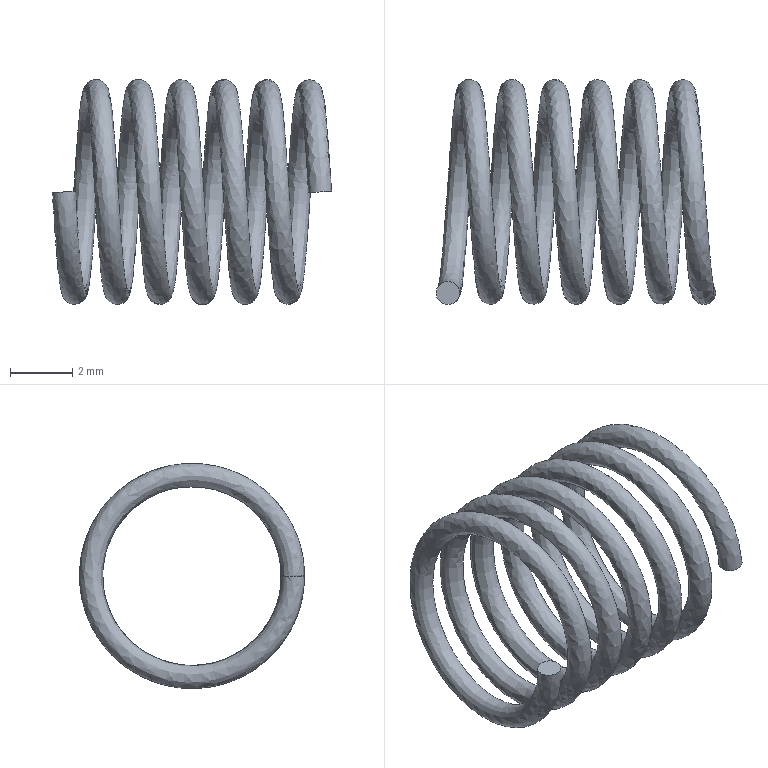Part | STEP file | 1-30.2 | 1 solid | 3 faces | box 8.998 x 7.25 x 7.252 mm | volume 54.263 mm3 | plane 2 | spline 1